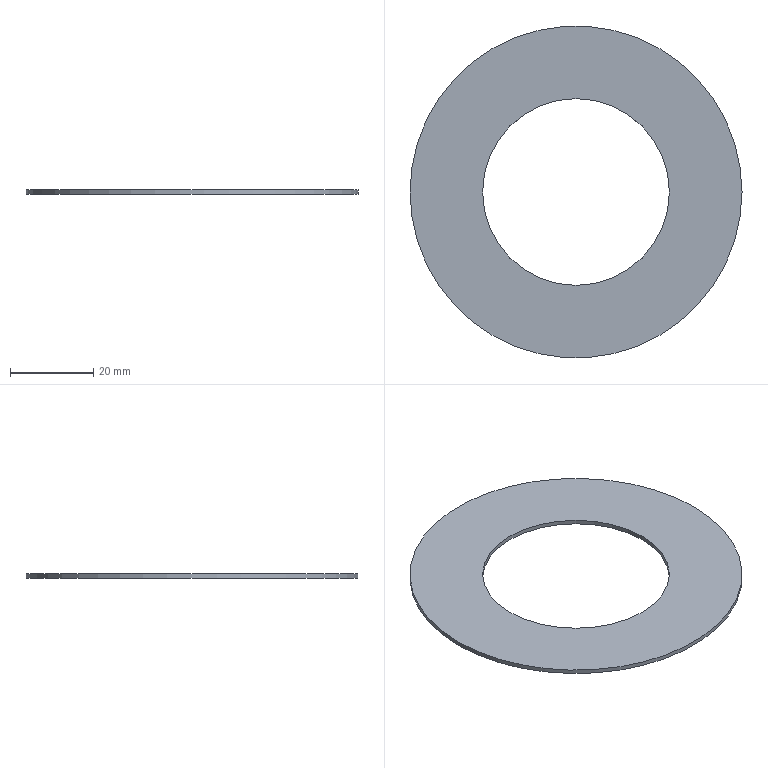Part | NX | features solid 2 | 1 solid | 4 faces | box 80 x 80 x 1 mm | volume 3436 mm3 | cylinder 2 | plane 2 | commonest cylinder face diameters 45 x1 80 x1
STEP:
#1=CARTESIAN_POINT('',(148.036,189.417,1.));
#2=VERTEX_POINT('',#1);
#3=CARTESIAN_POINT('',(108.036,189.417,1.));
#4=DIRECTION('',(0.,0.,1.));
#5=DIRECTION('',(1.,0.,0.));
#6=AXIS2_PLACEMENT_3D('',#3,#4,#5);
#7=CIRCLE('',#6,40.);
#8=EDGE_CURVE('',#2,#2,#7,.T.);
#9=ORIENTED_EDGE('',*,*,#8,.F.);
#10=EDGE_LOOP('',(#9));
#11=FACE_BOUND('',#10,.T.);
#12=CARTESIAN_POINT('',(148.036,189.417,0.));
#13=VERTEX_POINT('',#12);
#14=CARTESIAN_POINT('',(108.036,189.417,0.));
#15=DIRECTION('',(0.,0.,1.));
#16=DIRECTION('',(1.,0.,0.));
#17=AXIS2_PLACEMENT_3D('',#14,#15,#16);
#18=CIRCLE('',#17,40.);
#19=EDGE_CURVE('',#13,#13,#18,.T.);
#20=ORIENTED_EDGE('',*,*,#19,.T.);
#21=EDGE_LOOP('',(#20));
#22=FACE_BOUND('',#21,.T.);
#23=CARTESIAN_POINT('',(108.036,189.417,1.));
#24=DIRECTION('',(0.,0.,-1.));
#25=DIRECTION('',(-1.,0.,0.));
#26=AXIS2_PLACEMENT_3D('',#23,#24,#25);
#27=CYLINDRICAL_SURFACE('',#26,40.);
#28=ADVANCED_FACE('',(#11,#22),#27,.T.);
#29=CARTESIAN_POINT('',(130.536,189.417,1.));
#30=VERTEX_POINT('',#29);
#31=CARTESIAN_POINT('',(108.036,189.417,1.));
#32=DIRECTION('',(0.,0.,1.));
#33=DIRECTION('',(1.,0.,0.));
#34=AXIS2_PLACEMENT_3D('',#31,#32,#33);
#35=CIRCLE('',#34,22.5);
#36=EDGE_CURVE('',#30,#30,#35,.T.);
#37=ORIENTED_EDGE('',*,*,#36,.T.);
#38=EDGE_LOOP('',(#37));
#39=FACE_BOUND('',#38,.T.);
#40=CARTESIAN_POINT('',(130.536,189.417,0.));
#41=VERTEX_POINT('',#40);
#42=CARTESIAN_POINT('',(108.036,189.417,0.));
#43=DIRECTION('',(0.,0.,1.));
#44=DIRECTION('',(1.,0.,0.));
#45=AXIS2_PLACEMENT_3D('',#42,#43,#44);
#46=CIRCLE('',#45,22.5);
#47=EDGE_CURVE('',#41,#41,#46,.T.);
#48=ORIENTED_EDGE('',*,*,#47,.F.);
#49=EDGE_LOOP('',(#48));
#50=FACE_BOUND('',#49,.T.);
#51=CARTESIAN_POINT('',(108.036,189.417,1.));
#52=DIRECTION('',(0.,0.,-1.));
#53=DIRECTION('',(-1.,0.,0.));
#54=AXIS2_PLACEMENT_3D('',#51,#52,#53);
#55=CYLINDRICAL_SURFACE('',#54,22.5);
#56=ADVANCED_FACE('',(#39,#50),#55,.F.);
#57=ORIENTED_EDGE('',*,*,#8,.T.);
#58=EDGE_LOOP('',(#57));
#59=FACE_BOUND('',#58,.T.);
#60=ORIENTED_EDGE('',*,*,#36,.F.);
#61=EDGE_LOOP('',(#60));
#62=FACE_BOUND('',#61,.T.);
#63=CARTESIAN_POINT('',(108.036,189.417,1.));
#64=DIRECTION('',(0.,0.,1.));
#65=DIRECTION('',(1.,0.,0.));
#66=AXIS2_PLACEMENT_3D('',#63,#64,#65);
#67=PLANE('',#66);
#68=ADVANCED_FACE('',(#59,#62),#67,.T.);
#69=ORIENTED_EDGE('',*,*,#19,.F.);
#70=EDGE_LOOP('',(#69));
#71=FACE_BOUND('',#70,.T.);
#72=ORIENTED_EDGE('',*,*,#47,.T.);
#73=EDGE_LOOP('',(#72));
#74=FACE_BOUND('',#73,.T.);
#75=CARTESIAN_POINT('',(108.036,189.417,0.));
#76=DIRECTION('',(0.,0.,1.));
#77=DIRECTION('',(1.,0.,0.));
#78=AXIS2_PLACEMENT_3D('',#75,#76,#77);
#79=PLANE('',#78);
#80=ADVANCED_FACE('',(#71,#74),#79,.F.);
#81=CLOSED_SHELL('',(#28,#56,#68,#80));
#82=MANIFOLD_SOLID_BREP('',#81);
#83=(LENGTH_UNIT()NAMED_UNIT(*)SI_UNIT(.MILLI.,.METRE.));
#84=UNCERTAINTY_MEASURE_WITH_UNIT(LENGTH_MEASURE(0.00001),#83,'','');
#85=(NAMED_UNIT(*)PLANE_ANGLE_UNIT()SI_UNIT($,.RADIAN.));
#86=(NAMED_UNIT(*)SI_UNIT($,.STERADIAN.)SOLID_ANGLE_UNIT());
#87=(GEOMETRIC_REPRESENTATION_CONTEXT(3)GLOBAL_UNCERTAINTY_ASSIGNED_CONTEXT((#84))GLOBAL_UNIT_ASSIGNED_CONTEXT((#83,#85,#86))REPRESENTATION_CONTEXT('',''));
#88=ADVANCED_BREP_SHAPE_REPRESENTATION('',(#82),#87);